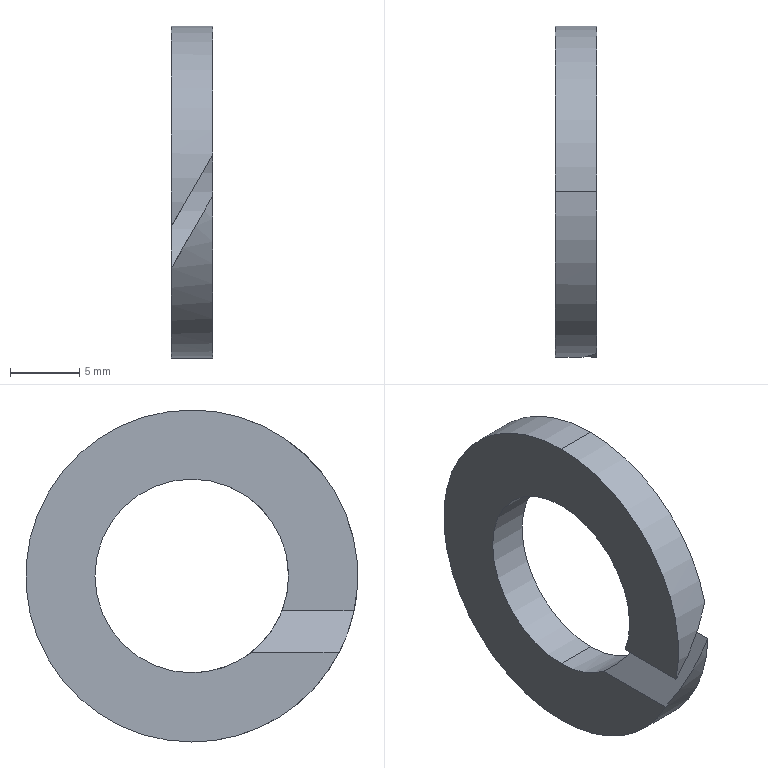Part | SolidWorks | features ICE 1, Revolution 1 | 1 solid | 10 faces | box 3 x 24 x 24 mm | volume 848.529 mm3 | cylinder 6 | plane 4 | commonest cylinder face diameters 14 x3 24 x3
STEP:
#1=CARTESIAN_POINT('',(15.483,0.,-7.));
#2=VERTEX_POINT('',#1);
#3=CARTESIAN_POINT('',(15.483,-6.995,-0.274));
#4=VERTEX_POINT('',#3);
#5=CARTESIAN_POINT('',(15.483,0.,0.));
#6=DIRECTION('',(-1.,0.,0.));
#7=DIRECTION('',(0.,0.,1.));
#8=AXIS2_PLACEMENT_3D('',#5,#6,#7);
#9=CIRCLE('',#8,7.);
#10=EDGE_CURVE('',#2,#4,#9,.T.);
#11=ORIENTED_EDGE('',*,*,#10,.F.);
#12=CARTESIAN_POINT('',(12.483,0.,-7.));
#13=VERTEX_POINT('',#12);
#14=CARTESIAN_POINT('',(0.,0.,-7.));
#15=DIRECTION('',(-1.,0.,0.));
#16=VECTOR('',#15,1000.);
#17=LINE('',#14,#16);
#18=EDGE_CURVE('',#2,#13,#17,.T.);
#19=ORIENTED_EDGE('',*,*,#18,.T.);
#20=CARTESIAN_POINT('',(12.483,-4.299,-5.524));
#21=VERTEX_POINT('',#20);
#22=CARTESIAN_POINT('',(12.483,0.,0.));
#23=DIRECTION('',(-1.,0.,0.));
#24=DIRECTION('',(0.,0.,1.));
#25=AXIS2_PLACEMENT_3D('',#22,#23,#24);
#26=CIRCLE('',#25,7.);
#27=EDGE_CURVE('',#13,#21,#26,.T.);
#28=ORIENTED_EDGE('',*,*,#27,.T.);
#29=CARTESIAN_POINT('',(15.483,-6.995,-0.274));
#30=CARTESIAN_POINT('',(14.285,-6.913,-2.37));
#31=CARTESIAN_POINT('',(13.219,-5.955,-4.236));
#32=CARTESIAN_POINT('',(12.483,-4.299,-5.524));
#33=(BOUNDED_CURVE()B_SPLINE_CURVE(3,(#29,#30,#31,#32),.UNSPECIFIED.,.F.,.F.)B_SPLINE_CURVE_WITH_KNOTS((4,4),(4.752,5.622),.UNSPECIFIED.)CURVE()GEOMETRIC_REPRESENTATION_ITEM()RATIONAL_B_SPLINE_CURVE((1.,0.9379,0.9379,1.))REPRESENTATION_ITEM(''));
#34=EDGE_CURVE('',#4,#21,#33,.T.);
#35=ORIENTED_EDGE('',*,*,#34,.F.);
#36=EDGE_LOOP('',(#11,#19,#28,#35));
#37=FACE_OUTER_BOUND('',#36,.T.);
#38=CARTESIAN_POINT('',(0.,0.,0.));
#39=DIRECTION('',(-1.,0.,0.));
#40=DIRECTION('',(0.,0.,1.));
#41=AXIS2_PLACEMENT_3D('',#38,#39,#40);
#42=CYLINDRICAL_SURFACE('',#41,7.);
#43=ADVANCED_FACE('',(#37),#42,.F.);
#44=ORIENTED_EDGE('',*,*,#18,.F.);
#45=CARTESIAN_POINT('',(15.483,0.,7.));
#46=VERTEX_POINT('',#45);
#47=CARTESIAN_POINT('',(15.483,0.,0.));
#48=DIRECTION('',(-1.,0.,0.));
#49=DIRECTION('',(0.,0.,1.));
#50=AXIS2_PLACEMENT_3D('',#47,#48,#49);
#51=CIRCLE('',#50,7.);
#52=EDGE_CURVE('',#46,#2,#51,.T.);
#53=ORIENTED_EDGE('',*,*,#52,.F.);
#54=CARTESIAN_POINT('',(12.483,0.,7.));
#55=VERTEX_POINT('',#54);
#56=CARTESIAN_POINT('',(0.,0.,7.));
#57=DIRECTION('',(-1.,0.,0.));
#58=VECTOR('',#57,1000.);
#59=LINE('',#56,#58);
#60=EDGE_CURVE('',#46,#55,#59,.T.);
#61=ORIENTED_EDGE('',*,*,#60,.T.);
#62=CARTESIAN_POINT('',(12.483,0.,0.));
#63=DIRECTION('',(-1.,0.,0.));
#64=DIRECTION('',(0.,0.,1.));
#65=AXIS2_PLACEMENT_3D('',#62,#63,#64);
#66=CIRCLE('',#65,7.);
#67=EDGE_CURVE('',#55,#13,#66,.T.);
#68=ORIENTED_EDGE('',*,*,#67,.T.);
#69=EDGE_LOOP('',(#44,#53,#61,#68));
#70=FACE_OUTER_BOUND('',#69,.T.);
#71=CARTESIAN_POINT('',(0.,0.,0.));
#72=DIRECTION('',(-1.,0.,0.));
#73=DIRECTION('',(0.,0.,1.));
#74=AXIS2_PLACEMENT_3D('',#71,#72,#73);
#75=CYLINDRICAL_SURFACE('',#74,7.);
#76=ADVANCED_FACE('',(#70),#75,.F.);
#77=CARTESIAN_POINT('',(15.483,0.,12.));
#78=VERTEX_POINT('',#77);
#79=CARTESIAN_POINT('',(15.483,0.,-12.));
#80=VERTEX_POINT('',#79);
#81=CARTESIAN_POINT('',(15.483,0.,0.));
#82=DIRECTION('',(-1.,0.,0.));
#83=DIRECTION('',(0.,0.,1.));
#84=AXIS2_PLACEMENT_3D('',#81,#82,#83);
#85=CIRCLE('',#84,12.);
#86=EDGE_CURVE('',#78,#80,#85,.T.);
#87=ORIENTED_EDGE('',*,*,#86,.T.);
#88=CARTESIAN_POINT('',(12.483,0.,-12.));
#89=VERTEX_POINT('',#88);
#90=CARTESIAN_POINT('',(0.,0.,-12.));
#91=DIRECTION('',(-1.,0.,0.));
#92=VECTOR('',#91,1000.);
#93=LINE('',#90,#92);
#94=EDGE_CURVE('',#80,#89,#93,.T.);
#95=ORIENTED_EDGE('',*,*,#94,.T.);
#96=CARTESIAN_POINT('',(12.483,0.,12.));
#97=VERTEX_POINT('',#96);
#98=CARTESIAN_POINT('',(12.483,0.,0.));
#99=DIRECTION('',(-1.,0.,0.));
#100=DIRECTION('',(0.,0.,1.));
#101=AXIS2_PLACEMENT_3D('',#98,#99,#100);
#102=CIRCLE('',#101,12.);
#103=EDGE_CURVE('',#97,#89,#102,.T.);
#104=ORIENTED_EDGE('',*,*,#103,.F.);
#105=CARTESIAN_POINT('',(0.,0.,12.));
#106=DIRECTION('',(-1.,0.,0.));
#107=VECTOR('',#106,1000.);
#108=LINE('',#105,#107);
#109=EDGE_CURVE('',#78,#97,#108,.T.);
#110=ORIENTED_EDGE('',*,*,#109,.F.);
#111=EDGE_LOOP('',(#87,#95,#104,#110));
#112=FACE_OUTER_BOUND('',#111,.T.);
#113=CARTESIAN_POINT('',(0.,0.,0.));
#114=DIRECTION('',(-1.,0.,0.));
#115=DIRECTION('',(0.,0.,1.));
#116=AXIS2_PLACEMENT_3D('',#113,#114,#115);
#117=CYLINDRICAL_SURFACE('',#116,12.);
#118=ADVANCED_FACE('',(#112),#117,.T.);
#119=CARTESIAN_POINT('',(15.483,-11.682,2.745));
#120=VERTEX_POINT('',#119);
#121=CARTESIAN_POINT('',(15.483,0.,0.));
#122=DIRECTION('',(-1.,0.,0.));
#123=DIRECTION('',(0.,0.,1.));
#124=AXIS2_PLACEMENT_3D('',#121,#122,#123);
#125=CIRCLE('',#124,12.);
#126=EDGE_CURVE('',#120,#78,#125,.T.);
#127=ORIENTED_EDGE('',*,*,#126,.T.);
#128=ORIENTED_EDGE('',*,*,#109,.T.);
#129=CARTESIAN_POINT('',(12.483,-11.736,-2.505));
#130=VERTEX_POINT('',#129);
#131=CARTESIAN_POINT('',(12.483,0.,0.));
#132=DIRECTION('',(-1.,0.,0.));
#133=DIRECTION('',(0.,0.,1.));
#134=AXIS2_PLACEMENT_3D('',#131,#132,#133);
#135=CIRCLE('',#134,12.);
#136=EDGE_CURVE('',#130,#97,#135,.T.);
#137=ORIENTED_EDGE('',*,*,#136,.F.);
#138=CARTESIAN_POINT('',(15.483,-11.682,2.745));
#139=CARTESIAN_POINT('',(14.493,-12.089,1.013));
#140=CARTESIAN_POINT('',(13.477,-12.107,-0.7658));
#141=CARTESIAN_POINT('',(12.483,-11.736,-2.505));
#142=(BOUNDED_CURVE()B_SPLINE_CURVE(3,(#138,#139,#140,#141),.UNSPECIFIED.,.F.,.T.)B_SPLINE_CURVE_WITH_KNOTS((4,4),(4.482,4.923),.UNSPECIFIED.)CURVE()GEOMETRIC_REPRESENTATION_ITEM()RATIONAL_B_SPLINE_CURVE((1.,0.9839,0.9839,1.))REPRESENTATION_ITEM(''));
#143=EDGE_CURVE('',#120,#130,#142,.T.);
#144=ORIENTED_EDGE('',*,*,#143,.F.);
#145=EDGE_LOOP('',(#127,#128,#137,#144));
#146=FACE_OUTER_BOUND('',#145,.T.);
#147=CARTESIAN_POINT('',(0.,0.,0.));
#148=DIRECTION('',(-1.,0.,0.));
#149=DIRECTION('',(0.,0.,1.));
#150=AXIS2_PLACEMENT_3D('',#147,#148,#149);
#151=CYLINDRICAL_SURFACE('',#150,12.);
#152=ADVANCED_FACE('',(#146),#151,.T.);
#153=CARTESIAN_POINT('',(12.483,-6.536,-2.505));
#154=VERTEX_POINT('',#153);
#155=CARTESIAN_POINT('',(12.483,0.,0.));
#156=DIRECTION('',(-1.,0.,0.));
#157=DIRECTION('',(0.,0.,1.));
#158=AXIS2_PLACEMENT_3D('',#155,#156,#157);
#159=CIRCLE('',#158,7.);
#160=EDGE_CURVE('',#154,#55,#159,.T.);
#161=ORIENTED_EDGE('',*,*,#160,.F.);
#162=CARTESIAN_POINT('',(12.483,-12.001,-2.505));
#163=DIRECTION('',(0.,1.,0.));
#164=VECTOR('',#163,1000.);
#165=LINE('',#162,#164);
#166=EDGE_CURVE('',#130,#154,#165,.T.);
#167=ORIENTED_EDGE('',*,*,#166,.F.);
#168=ORIENTED_EDGE('',*,*,#136,.T.);
#169=ORIENTED_EDGE('',*,*,#103,.T.);
#170=CARTESIAN_POINT('',(12.483,-10.653,-5.524));
#171=VERTEX_POINT('',#170);
#172=CARTESIAN_POINT('',(12.483,0.,0.));
#173=DIRECTION('',(-1.,0.,0.));
#174=DIRECTION('',(0.,0.,1.));
#175=AXIS2_PLACEMENT_3D('',#172,#173,#174);
#176=CIRCLE('',#175,12.);
#177=EDGE_CURVE('',#89,#171,#176,.T.);
#178=ORIENTED_EDGE('',*,*,#177,.T.);
#179=CARTESIAN_POINT('',(12.483,-12.001,-5.524));
#180=DIRECTION('',(0.,-1.,0.));
#181=VECTOR('',#180,1000.);
#182=LINE('',#179,#181);
#183=EDGE_CURVE('',#21,#171,#182,.T.);
#184=ORIENTED_EDGE('',*,*,#183,.F.);
#185=ORIENTED_EDGE('',*,*,#27,.F.);
#186=ORIENTED_EDGE('',*,*,#67,.F.);
#187=EDGE_LOOP('',(#161,#167,#168,#169,#178,#184,#185,#186));
#188=FACE_OUTER_BOUND('',#187,.T.);
#189=CARTESIAN_POINT('',(12.483,7.,0.));
#190=DIRECTION('',(1.,0.,0.));
#191=DIRECTION('',(0.,0.,-1.));
#192=AXIS2_PLACEMENT_3D('',#189,#190,#191);
#193=PLANE('',#192);
#194=ADVANCED_FACE('',(#188),#193,.F.);
#195=ORIENTED_EDGE('',*,*,#94,.F.);
#196=CARTESIAN_POINT('',(15.483,-11.997,-0.274));
#197=VERTEX_POINT('',#196);
#198=CARTESIAN_POINT('',(15.483,0.,0.));
#199=DIRECTION('',(-1.,0.,0.));
#200=DIRECTION('',(0.,0.,1.));
#201=AXIS2_PLACEMENT_3D('',#198,#199,#200);
#202=CIRCLE('',#201,12.);
#203=EDGE_CURVE('',#80,#197,#202,.T.);
#204=ORIENTED_EDGE('',*,*,#203,.T.);
#205=CARTESIAN_POINT('',(12.483,-10.653,-5.524));
#206=CARTESIAN_POINT('',(13.415,-11.499,-3.892));
#207=CARTESIAN_POINT('',(14.433,-11.955,-2.112));
#208=CARTESIAN_POINT('',(15.483,-11.997,-0.274));
#209=(BOUNDED_CURVE()B_SPLINE_CURVE(3,(#205,#206,#207,#208),.UNSPECIFIED.,.F.,.F.)B_SPLINE_CURVE_WITH_KNOTS((4,4),(1.092,1.548),.UNSPECIFIED.)CURVE()GEOMETRIC_REPRESENTATION_ITEM()RATIONAL_B_SPLINE_CURVE((1.,0.9828,0.9828,1.))REPRESENTATION_ITEM(''));
#210=EDGE_CURVE('',#171,#197,#209,.T.);
#211=ORIENTED_EDGE('',*,*,#210,.F.);
#212=ORIENTED_EDGE('',*,*,#177,.F.);
#213=EDGE_LOOP('',(#195,#204,#211,#212));
#214=FACE_OUTER_BOUND('',#213,.T.);
#215=CARTESIAN_POINT('',(0.,0.,0.));
#216=DIRECTION('',(-1.,0.,0.));
#217=DIRECTION('',(0.,0.,1.));
#218=AXIS2_PLACEMENT_3D('',#215,#216,#217);
#219=CYLINDRICAL_SURFACE('',#218,12.);
#220=ADVANCED_FACE('',(#214),#219,.T.);
#221=ORIENTED_EDGE('',*,*,#126,.F.);
#222=CARTESIAN_POINT('',(15.483,-6.439,2.745));
#223=VERTEX_POINT('',#222);
#224=CARTESIAN_POINT('',(15.483,-12.001,2.745));
#225=DIRECTION('',(0.,-1.,0.));
#226=VECTOR('',#225,1000.);
#227=LINE('',#224,#226);
#228=EDGE_CURVE('',#223,#120,#227,.T.);
#229=ORIENTED_EDGE('',*,*,#228,.F.);
#230=CARTESIAN_POINT('',(15.483,0.,0.));
#231=DIRECTION('',(-1.,0.,0.));
#232=DIRECTION('',(0.,0.,1.));
#233=AXIS2_PLACEMENT_3D('',#230,#231,#232);
#234=CIRCLE('',#233,7.);
#235=EDGE_CURVE('',#223,#46,#234,.T.);
#236=ORIENTED_EDGE('',*,*,#235,.T.);
#237=ORIENTED_EDGE('',*,*,#52,.T.);
#238=ORIENTED_EDGE('',*,*,#10,.T.);
#239=CARTESIAN_POINT('',(15.483,-12.001,-0.274));
#240=DIRECTION('',(0.,1.,0.));
#241=VECTOR('',#240,1000.);
#242=LINE('',#239,#241);
#243=EDGE_CURVE('',#197,#4,#242,.T.);
#244=ORIENTED_EDGE('',*,*,#243,.F.);
#245=ORIENTED_EDGE('',*,*,#203,.F.);
#246=ORIENTED_EDGE('',*,*,#86,.F.);
#247=EDGE_LOOP('',(#221,#229,#236,#237,#238,#244,#245,#246));
#248=FACE_OUTER_BOUND('',#247,.T.);
#249=CARTESIAN_POINT('',(15.483,7.,0.));
#250=DIRECTION('',(-1.,0.,0.));
#251=DIRECTION('',(0.,0.,1.));
#252=AXIS2_PLACEMENT_3D('',#249,#250,#251);
#253=PLANE('',#252);
#254=ADVANCED_FACE('',(#248),#253,.F.);
#255=ORIENTED_EDGE('',*,*,#60,.F.);
#256=ORIENTED_EDGE('',*,*,#235,.F.);
#257=CARTESIAN_POINT('',(12.483,-6.536,-2.505));
#258=CARTESIAN_POINT('',(13.464,-7.195,-0.7874));
#259=CARTESIAN_POINT('',(14.515,-7.161,1.052));
#260=CARTESIAN_POINT('',(15.483,-6.439,2.745));
#261=(BOUNDED_CURVE()B_SPLINE_CURVE(3,(#257,#258,#259,#260),.UNSPECIFIED.,.F.,.F.)B_SPLINE_CURVE_WITH_KNOTS((4,4),(1.205,1.974),.UNSPECIFIED.)CURVE()GEOMETRIC_REPRESENTATION_ITEM()RATIONAL_B_SPLINE_CURVE((1.,0.9513,0.9513,1.))REPRESENTATION_ITEM(''));
#262=EDGE_CURVE('',#154,#223,#261,.T.);
#263=ORIENTED_EDGE('',*,*,#262,.F.);
#264=ORIENTED_EDGE('',*,*,#160,.T.);
#265=EDGE_LOOP('',(#255,#256,#263,#264));
#266=FACE_OUTER_BOUND('',#265,.T.);
#267=CARTESIAN_POINT('',(0.,0.,0.));
#268=DIRECTION('',(-1.,0.,0.));
#269=DIRECTION('',(0.,0.,1.));
#270=AXIS2_PLACEMENT_3D('',#267,#268,#269);
#271=CYLINDRICAL_SURFACE('',#270,7.);
#272=ADVANCED_FACE('',(#266),#271,.F.);
#273=ORIENTED_EDGE('',*,*,#183,.T.);
#274=ORIENTED_EDGE('',*,*,#210,.T.);
#275=ORIENTED_EDGE('',*,*,#243,.T.);
#276=ORIENTED_EDGE('',*,*,#34,.T.);
#277=EDGE_LOOP('',(#273,#274,#275,#276));
#278=FACE_OUTER_BOUND('',#277,.T.);
#279=CARTESIAN_POINT('',(7.695,-12.001,-13.903));
#280=DIRECTION('',(0.8682,0.,-0.4961));
#281=DIRECTION('',(-0.4961,0.,-0.8682));
#282=AXIS2_PLACEMENT_3D('',#279,#280,#281);
#283=PLANE('',#282);
#284=ADVANCED_FACE('',(#278),#283,.F.);
#285=ORIENTED_EDGE('',*,*,#166,.T.);
#286=ORIENTED_EDGE('',*,*,#262,.T.);
#287=ORIENTED_EDGE('',*,*,#228,.T.);
#288=ORIENTED_EDGE('',*,*,#143,.T.);
#289=EDGE_LOOP('',(#285,#286,#287,#288));
#290=FACE_OUTER_BOUND('',#289,.T.);
#291=CARTESIAN_POINT('',(22.653,-12.001,15.293));
#292=DIRECTION('',(-0.8682,0.,0.4961));
#293=DIRECTION('',(0.4961,0.,0.8682));
#294=AXIS2_PLACEMENT_3D('',#291,#292,#293);
#295=PLANE('',#294);
#296=ADVANCED_FACE('',(#290),#295,.F.);
#297=CLOSED_SHELL('',(#43,#76,#118,#152,#194,#220,#254,#272,#284,#296));
#298=MANIFOLD_SOLID_BREP('',#297);
#299=CARTESIAN_POINT('',(0.,0.,0.));
#300=DIRECTION('',(0.,0.,1.));
#301=DIRECTION('',(1.,0.,0.));
#302=AXIS2_PLACEMENT_3D('',#299,#300,#301);
#303=(LENGTH_UNIT()NAMED_UNIT(*)SI_UNIT(.MILLI.,.METRE.));
#304=UNCERTAINTY_MEASURE_WITH_UNIT(LENGTH_MEASURE(0.00001),#303,'','');
#305=(NAMED_UNIT(*)PLANE_ANGLE_UNIT()SI_UNIT($,.RADIAN.));
#306=(NAMED_UNIT(*)SI_UNIT($,.STERADIAN.)SOLID_ANGLE_UNIT());
#307=(GEOMETRIC_REPRESENTATION_CONTEXT(3)GLOBAL_UNCERTAINTY_ASSIGNED_CONTEXT((#304))GLOBAL_UNIT_ASSIGNED_CONTEXT((#303,#305,#306))REPRESENTATION_CONTEXT('',''));
#308=ADVANCED_BREP_SHAPE_REPRESENTATION('',(#298,#302),#307);